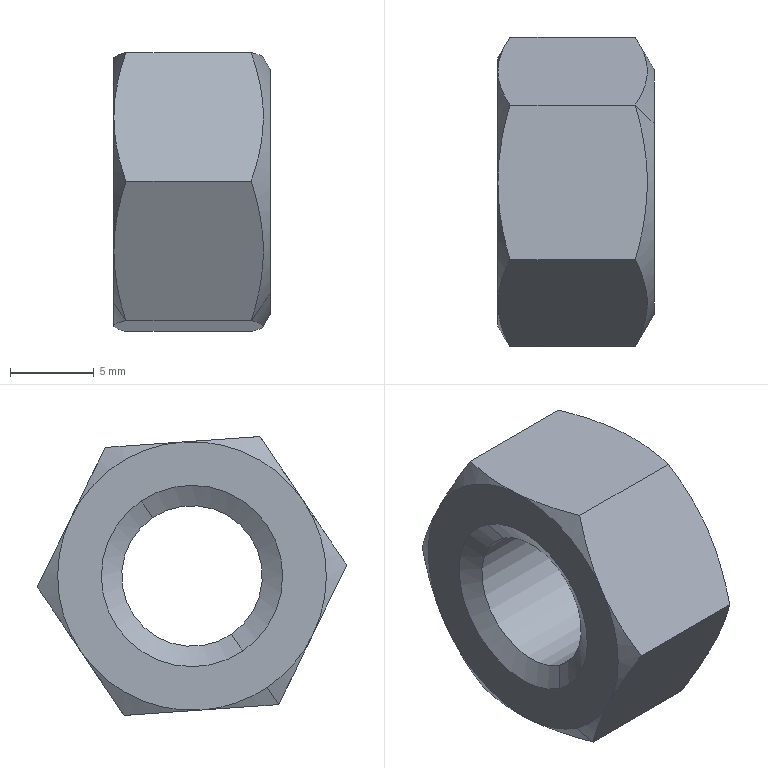Part | NX | features BREP 1 | 1 solid | 23 faces | box 9.3 x 18.43 x 16.607 mm | volume 1512 mm3 | cone 13 | plane 8 | cylinder 2 | commonest cylinder face diameters 8.376 x2
STEP:
#1=CARTESIAN_POINT('',(711.535,38.26,-40.972));
#2=VERTEX_POINT('',#1);
#3=CARTESIAN_POINT('',(711.535,33.574,-47.915));
#4=VERTEX_POINT('',#3);
#5=CARTESIAN_POINT('',(711.535,35.917,-44.443));
#6=DIRECTION('',(1.,0.,0.));
#7=DIRECTION('',(0.,-0.5594,-0.8289));
#8=AXIS2_PLACEMENT_3D('',#5,#6,#7);
#9=CIRCLE('',#8,4.188);
#10=EDGE_CURVE('',#2,#4,#9,.T.);
#11=ORIENTED_EDGE('',*,*,#10,.F.);
#12=CARTESIAN_POINT('',(711.845,38.433,-40.715));
#13=VERTEX_POINT('',#12);
#14=CARTESIAN_POINT('',(711.535,38.26,-40.972));
#15=DIRECTION('',(0.7071,0.3956,0.5861));
#16=VECTOR('',#15,1000.);
#17=LINE('',#14,#16);
#18=EDGE_CURVE('',#13,#2,#17,.F.);
#19=ORIENTED_EDGE('',*,*,#18,.F.);
#20=CARTESIAN_POINT('',(711.845,33.401,-48.172));
#21=VERTEX_POINT('',#20);
#22=CARTESIAN_POINT('',(711.845,35.917,-44.443));
#23=DIRECTION('',(-1.,0.,0.));
#24=DIRECTION('',(0.,-0.5594,-0.8289));
#25=AXIS2_PLACEMENT_3D('',#22,#23,#24);
#26=CIRCLE('',#25,4.498);
#27=EDGE_CURVE('',#21,#13,#26,.T.);
#28=ORIENTED_EDGE('',*,*,#27,.F.);
#29=CARTESIAN_POINT('',(711.535,33.574,-47.915));
#30=DIRECTION('',(0.7071,-0.3956,-0.5861));
#31=VECTOR('',#30,1000.);
#32=LINE('',#29,#31);
#33=EDGE_CURVE('',#21,#4,#32,.F.);
#34=ORIENTED_EDGE('',*,*,#33,.T.);
#35=EDGE_LOOP('',(#11,#19,#28,#34));
#36=FACE_BOUND('',#35,.T.);
#37=CARTESIAN_POINT('',(711.535,35.917,-44.443));
#38=DIRECTION('',(1.,0.,0.));
#39=DIRECTION('',(0.,0.5594,0.8289));
#40=AXIS2_PLACEMENT_3D('',#37,#38,#39);
#41=CONICAL_SURFACE('',#40,4.188,0.7854);
#42=ADVANCED_FACE('',(#36),#41,.F.);
#43=CARTESIAN_POINT('',(711.845,40.001,-38.392));
#44=VERTEX_POINT('',#43);
#45=CARTESIAN_POINT('',(711.845,31.834,-50.494));
#46=VERTEX_POINT('',#45);
#47=CARTESIAN_POINT('',(711.845,35.917,-44.443));
#48=DIRECTION('',(-1.,0.,0.));
#49=DIRECTION('',(0.,0.5594,0.8289));
#50=AXIS2_PLACEMENT_3D('',#47,#48,#49);
#51=CIRCLE('',#50,7.3);
#52=EDGE_CURVE('',#44,#46,#51,.T.);
#53=ORIENTED_EDGE('',*,*,#52,.T.);
#54=CARTESIAN_POINT('',(710.726,30.75,-52.1));
#55=VERTEX_POINT('',#54);
#56=CARTESIAN_POINT('',(710.726,30.75,-52.1));
#57=DIRECTION('',(-0.5,-0.4845,-0.7178));
#58=VECTOR('',#57,1000.);
#59=LINE('',#56,#58);
#60=EDGE_CURVE('',#46,#55,#59,.T.);
#61=ORIENTED_EDGE('',*,*,#60,.T.);
#62=CARTESIAN_POINT('',(710.726,39.965,-52.747));
#63=VERTEX_POINT('',#62);
#64=CARTESIAN_POINT('',(710.726,39.965,-52.747));
#65=CARTESIAN_POINT('',(711.162,38.46,-52.641));
#66=CARTESIAN_POINT('',(711.72,35.374,-52.425));
#67=CARTESIAN_POINT('',(711.162,32.256,-52.206));
#68=CARTESIAN_POINT('',(710.726,30.75,-52.1));
#69=B_SPLINE_CURVE_WITH_KNOTS('',3,(#64,#65,#66,#67,#68),.UNSPECIFIED.,.F.,.F.,(4,1,4),(0.,0.004665,0.009329),.UNSPECIFIED.);
#70=EDGE_CURVE('',#63,#55,#69,.T.);
#71=ORIENTED_EDGE('',*,*,#70,.F.);
#72=CARTESIAN_POINT('',(710.726,45.132,-45.09));
#73=VERTEX_POINT('',#72);
#74=CARTESIAN_POINT('',(710.726,45.132,-45.09));
#75=CARTESIAN_POINT('',(711.162,44.288,-46.34));
#76=CARTESIAN_POINT('',(711.72,42.558,-48.905));
#77=CARTESIAN_POINT('',(711.162,40.809,-51.495));
#78=CARTESIAN_POINT('',(710.726,39.965,-52.747));
#79=B_SPLINE_CURVE_WITH_KNOTS('',3,(#74,#75,#76,#77,#78),.UNSPECIFIED.,.F.,.F.,(4,1,4),(0.,0.004665,0.009329),.UNSPECIFIED.);
#80=EDGE_CURVE('',#73,#63,#79,.T.);
#81=ORIENTED_EDGE('',*,*,#80,.F.);
#82=CARTESIAN_POINT('',(710.726,41.085,-36.786));
#83=VERTEX_POINT('',#82);
#84=CARTESIAN_POINT('',(710.726,41.085,-36.786));
#85=CARTESIAN_POINT('',(711.162,41.746,-38.142));
#86=CARTESIAN_POINT('',(711.72,43.101,-40.923));
#87=CARTESIAN_POINT('',(711.162,44.47,-43.732));
#88=CARTESIAN_POINT('',(710.726,45.132,-45.09));
#89=B_SPLINE_CURVE_WITH_KNOTS('',3,(#84,#85,#86,#87,#88),.UNSPECIFIED.,.F.,.F.,(4,1,4),(0.,0.004665,0.009329),.UNSPECIFIED.);
#90=EDGE_CURVE('',#83,#73,#89,.T.);
#91=ORIENTED_EDGE('',*,*,#90,.F.);
#92=CARTESIAN_POINT('',(710.726,41.085,-36.786));
#93=DIRECTION('',(-0.5,0.4845,0.7178));
#94=VECTOR('',#93,1000.);
#95=LINE('',#92,#94);
#96=EDGE_CURVE('',#44,#83,#95,.T.);
#97=ORIENTED_EDGE('',*,*,#96,.F.);
#98=EDGE_LOOP('',(#53,#61,#71,#81,#91,#97));
#99=FACE_BOUND('',#98,.T.);
#100=CARTESIAN_POINT('',(710.726,35.917,-44.443));
#101=DIRECTION('',(-1.,0.,0.));
#102=DIRECTION('',(0.,-0.5594,-0.8289));
#103=AXIS2_PLACEMENT_3D('',#100,#101,#102);
#104=CONICAL_SURFACE('',#103,9.238,1.047);
#105=ADVANCED_FACE('',(#99),#104,.T.);
#106=CARTESIAN_POINT('',(703.245,38.26,-40.972));
#107=VERTEX_POINT('',#106);
#108=CARTESIAN_POINT('',(703.245,33.574,-47.915));
#109=VERTEX_POINT('',#108);
#110=CARTESIAN_POINT('',(703.245,35.917,-44.443));
#111=DIRECTION('',(1.,0.,0.));
#112=DIRECTION('',(0.,-0.5594,-0.8289));
#113=AXIS2_PLACEMENT_3D('',#110,#111,#112);
#114=CIRCLE('',#113,4.188);
#115=EDGE_CURVE('',#107,#109,#114,.T.);
#116=ORIENTED_EDGE('',*,*,#115,.T.);
#117=CARTESIAN_POINT('',(702.545,32.896,-48.919));
#118=VERTEX_POINT('',#117);
#119=CARTESIAN_POINT('',(703.245,33.574,-47.915));
#120=DIRECTION('',(-0.5,-0.4845,-0.7178));
#121=VECTOR('',#120,1000.);
#122=LINE('',#119,#121);
#123=EDGE_CURVE('',#109,#118,#122,.T.);
#124=ORIENTED_EDGE('',*,*,#123,.T.);
#125=CARTESIAN_POINT('',(702.545,38.938,-39.967));
#126=VERTEX_POINT('',#125);
#127=CARTESIAN_POINT('',(702.545,35.917,-44.443));
#128=DIRECTION('',(1.,0.,0.));
#129=DIRECTION('',(0.,-0.5594,-0.8289));
#130=AXIS2_PLACEMENT_3D('',#127,#128,#129);
#131=CIRCLE('',#130,5.4);
#132=EDGE_CURVE('',#126,#118,#131,.T.);
#133=ORIENTED_EDGE('',*,*,#132,.F.);
#134=CARTESIAN_POINT('',(703.245,38.26,-40.972));
#135=DIRECTION('',(-0.5,0.4845,0.7178));
#136=VECTOR('',#135,1000.);
#137=LINE('',#134,#136);
#138=EDGE_CURVE('',#107,#126,#137,.T.);
#139=ORIENTED_EDGE('',*,*,#138,.F.);
#140=EDGE_LOOP('',(#116,#124,#133,#139));
#141=FACE_BOUND('',#140,.T.);
#142=CARTESIAN_POINT('',(703.245,35.917,-44.443));
#143=DIRECTION('',(-1.,0.,0.));
#144=DIRECTION('',(0.,-0.5594,-0.8289));
#145=AXIS2_PLACEMENT_3D('',#142,#143,#144);
#146=CONICAL_SURFACE('',#145,4.188,1.047);
#147=ADVANCED_FACE('',(#141),#146,.F.);
#148=CARTESIAN_POINT('',(702.545,28.726,-47.948));
#149=VERTEX_POINT('',#148);
#150=CARTESIAN_POINT('',(702.545,31.442,-51.074));
#151=VERTEX_POINT('',#150);
#152=CARTESIAN_POINT('',(702.545,35.917,-44.443));
#153=DIRECTION('',(1.,0.,0.));
#154=DIRECTION('',(0.,-0.5594,-0.8289));
#155=AXIS2_PLACEMENT_3D('',#152,#153,#154);
#156=CIRCLE('',#155,8.);
#157=EDGE_CURVE('',#149,#151,#156,.T.);
#158=ORIENTED_EDGE('',*,*,#157,.T.);
#159=CARTESIAN_POINT('',(703.26,30.75,-52.1));
#160=VERTEX_POINT('',#159);
#161=CARTESIAN_POINT('',(703.26,30.75,-52.1));
#162=DIRECTION('',(0.5,-0.4845,-0.7178));
#163=VECTOR('',#162,1000.);
#164=LINE('',#161,#163);
#165=EDGE_CURVE('',#151,#160,#164,.T.);
#166=ORIENTED_EDGE('',*,*,#165,.T.);
#167=CARTESIAN_POINT('',(702.545,28.726,-47.948));
#168=CARTESIAN_POINT('',(702.545,29.417,-49.366));
#169=CARTESIAN_POINT('',(702.824,30.088,-50.744));
#170=CARTESIAN_POINT('',(703.26,30.75,-52.1));
#171=B_SPLINE_CURVE_WITH_KNOTS('',3,(#167,#168,#169,#170),.UNSPECIFIED.,.F.,.F.,(4,4),(0.,0.004674),.UNSPECIFIED.);
#172=EDGE_CURVE('',#149,#160,#171,.T.);
#173=ORIENTED_EDGE('',*,*,#172,.F.);
#174=EDGE_LOOP('',(#158,#166,#173));
#175=FACE_BOUND('',#174,.T.);
#176=CARTESIAN_POINT('',(703.26,35.917,-44.443));
#177=DIRECTION('',(1.,0.,0.));
#178=DIRECTION('',(0.,0.5594,0.8289));
#179=AXIS2_PLACEMENT_3D('',#176,#177,#178);
#180=CONICAL_SURFACE('',#179,9.238,1.047);
#181=ADVANCED_FACE('',(#175),#180,.T.);
#182=ORIENTED_EDGE('',*,*,#115,.F.);
#183=CARTESIAN_POINT('',(702.545,38.26,-40.972));
#184=DIRECTION('',(1.,0.,0.));
#185=VECTOR('',#184,1000.);
#186=LINE('',#183,#185);
#187=EDGE_CURVE('',#2,#107,#186,.F.);
#188=ORIENTED_EDGE('',*,*,#187,.F.);
#189=ORIENTED_EDGE('',*,*,#10,.T.);
#190=CARTESIAN_POINT('',(702.545,33.574,-47.915));
#191=DIRECTION('',(1.,0.,0.));
#192=VECTOR('',#191,1000.);
#193=LINE('',#190,#192);
#194=EDGE_CURVE('',#4,#109,#193,.F.);
#195=ORIENTED_EDGE('',*,*,#194,.T.);
#196=EDGE_LOOP('',(#182,#188,#189,#195));
#197=FACE_BOUND('',#196,.T.);
#198=CARTESIAN_POINT('',(702.545,35.917,-44.443));
#199=DIRECTION('',(1.,0.,0.));
#200=DIRECTION('',(0.,0.5594,0.8289));
#201=AXIS2_PLACEMENT_3D('',#198,#199,#200);
#202=CYLINDRICAL_SURFACE('',#201,4.188);
#203=ADVANCED_FACE('',(#197),#202,.F.);
#204=CARTESIAN_POINT('',(703.26,26.702,-43.797));
#205=VERTEX_POINT('',#204);
#206=CARTESIAN_POINT('',(710.726,26.702,-43.797));
#207=VERTEX_POINT('',#206);
#208=CARTESIAN_POINT('',(702.545,26.702,-43.797));
#209=DIRECTION('',(1.,0.,0.));
#210=VECTOR('',#209,1000.);
#211=LINE('',#208,#210);
#212=EDGE_CURVE('',#205,#207,#211,.T.);
#213=ORIENTED_EDGE('',*,*,#212,.T.);
#214=CARTESIAN_POINT('',(710.726,31.87,-36.14));
#215=VERTEX_POINT('',#214);
#216=CARTESIAN_POINT('',(710.726,26.702,-43.797));
#217=CARTESIAN_POINT('',(711.162,27.546,-42.546));
#218=CARTESIAN_POINT('',(711.72,29.277,-39.982));
#219=CARTESIAN_POINT('',(711.162,31.025,-37.391));
#220=CARTESIAN_POINT('',(710.726,31.87,-36.14));
#221=B_SPLINE_CURVE_WITH_KNOTS('',3,(#216,#217,#218,#219,#220),.UNSPECIFIED.,.F.,.F.,(4,1,4),(0.,0.004665,0.009329),.UNSPECIFIED.);
#222=EDGE_CURVE('',#207,#215,#221,.T.);
#223=ORIENTED_EDGE('',*,*,#222,.T.);
#224=CARTESIAN_POINT('',(703.26,31.87,-36.14));
#225=VERTEX_POINT('',#224);
#226=CARTESIAN_POINT('',(702.545,31.87,-36.14));
#227=DIRECTION('',(1.,0.,0.));
#228=VECTOR('',#227,1000.);
#229=LINE('',#226,#228);
#230=EDGE_CURVE('',#225,#215,#229,.T.);
#231=ORIENTED_EDGE('',*,*,#230,.F.);
#232=CARTESIAN_POINT('',(702.545,29.286,-39.968));
#233=VERTEX_POINT('',#232);
#234=CARTESIAN_POINT('',(703.26,31.87,-36.14));
#235=CARTESIAN_POINT('',(702.824,31.026,-37.39));
#236=CARTESIAN_POINT('',(702.545,30.168,-38.661));
#237=CARTESIAN_POINT('',(702.545,29.286,-39.968));
#238=B_SPLINE_CURVE_WITH_KNOTS('',3,(#234,#235,#236,#237),.UNSPECIFIED.,.F.,.F.,(4,4),(0.,0.004674),.UNSPECIFIED.);
#239=EDGE_CURVE('',#225,#233,#238,.T.);
#240=ORIENTED_EDGE('',*,*,#239,.T.);
#241=CARTESIAN_POINT('',(702.545,29.286,-39.968));
#242=CARTESIAN_POINT('',(702.545,28.404,-41.275));
#243=CARTESIAN_POINT('',(702.824,27.546,-42.546));
#244=CARTESIAN_POINT('',(703.26,26.702,-43.797));
#245=B_SPLINE_CURVE_WITH_KNOTS('',3,(#241,#242,#243,#244),.UNSPECIFIED.,.F.,.F.,(4,4),(0.,0.004674),.UNSPECIFIED.);
#246=EDGE_CURVE('',#233,#205,#245,.T.);
#247=ORIENTED_EDGE('',*,*,#246,.T.);
#248=EDGE_LOOP('',(#213,#223,#231,#240,#247));
#249=FACE_BOUND('',#248,.T.);
#250=CARTESIAN_POINT('',(702.545,31.87,-36.14));
#251=DIRECTION('',(0.,-0.8289,0.5594));
#252=DIRECTION('',(1.,0.,0.));
#253=AXIS2_PLACEMENT_3D('',#250,#251,#252);
#254=PLANE('',#253);
#255=ADVANCED_FACE('',(#249),#254,.T.);
#256=ORIENTED_EDGE('',*,*,#230,.T.);
#257=CARTESIAN_POINT('',(710.726,31.87,-36.14));
#258=CARTESIAN_POINT('',(711.162,33.374,-36.245));
#259=CARTESIAN_POINT('',(711.72,36.461,-36.462));
#260=CARTESIAN_POINT('',(711.162,39.578,-36.681));
#261=CARTESIAN_POINT('',(710.726,41.085,-36.786));
#262=B_SPLINE_CURVE_WITH_KNOTS('',3,(#257,#258,#259,#260,#261),.UNSPECIFIED.,.F.,.F.,(4,1,4),(0.,0.004665,0.009329),.UNSPECIFIED.);
#263=EDGE_CURVE('',#215,#83,#262,.T.);
#264=ORIENTED_EDGE('',*,*,#263,.T.);
#265=CARTESIAN_POINT('',(703.26,41.085,-36.786));
#266=VERTEX_POINT('',#265);
#267=CARTESIAN_POINT('',(702.545,41.085,-36.786));
#268=DIRECTION('',(1.,0.,0.));
#269=VECTOR('',#268,1000.);
#270=LINE('',#267,#269);
#271=EDGE_CURVE('',#266,#83,#270,.T.);
#272=ORIENTED_EDGE('',*,*,#271,.F.);
#273=CARTESIAN_POINT('',(702.545,36.477,-36.463));
#274=VERTEX_POINT('',#273);
#275=CARTESIAN_POINT('',(703.26,41.085,-36.786));
#276=CARTESIAN_POINT('',(702.824,39.579,-36.681));
#277=CARTESIAN_POINT('',(702.545,38.05,-36.573));
#278=CARTESIAN_POINT('',(702.545,36.477,-36.463));
#279=B_SPLINE_CURVE_WITH_KNOTS('',3,(#275,#276,#277,#278),.UNSPECIFIED.,.F.,.F.,(4,4),(0.,0.004674),.UNSPECIFIED.);
#280=EDGE_CURVE('',#266,#274,#279,.T.);
#281=ORIENTED_EDGE('',*,*,#280,.T.);
#282=CARTESIAN_POINT('',(702.545,36.477,-36.463));
#283=CARTESIAN_POINT('',(702.545,34.905,-36.353));
#284=CARTESIAN_POINT('',(702.824,33.375,-36.245));
#285=CARTESIAN_POINT('',(703.26,31.87,-36.14));
#286=B_SPLINE_CURVE_WITH_KNOTS('',3,(#282,#283,#284,#285),.UNSPECIFIED.,.F.,.F.,(4,4),(0.,0.004674),.UNSPECIFIED.);
#287=EDGE_CURVE('',#274,#225,#286,.T.);
#288=ORIENTED_EDGE('',*,*,#287,.T.);
#289=EDGE_LOOP('',(#256,#264,#272,#281,#288));
#290=FACE_BOUND('',#289,.T.);
#291=CARTESIAN_POINT('',(702.545,41.085,-36.786));
#292=DIRECTION('',(0.,0.07,0.9975));
#293=DIRECTION('',(0.,0.9975,-0.07));
#294=AXIS2_PLACEMENT_3D('',#291,#292,#293);
#295=PLANE('',#294);
#296=ADVANCED_FACE('',(#290),#295,.T.);
#297=ORIENTED_EDGE('',*,*,#271,.T.);
#298=ORIENTED_EDGE('',*,*,#90,.T.);
#299=CARTESIAN_POINT('',(703.26,45.132,-45.09));
#300=VERTEX_POINT('',#299);
#301=CARTESIAN_POINT('',(702.545,45.132,-45.09));
#302=DIRECTION('',(1.,0.,0.));
#303=VECTOR('',#302,1000.);
#304=LINE('',#301,#303);
#305=EDGE_CURVE('',#300,#73,#304,.T.);
#306=ORIENTED_EDGE('',*,*,#305,.F.);
#307=CARTESIAN_POINT('',(702.545,43.108,-40.938));
#308=VERTEX_POINT('',#307);
#309=CARTESIAN_POINT('',(703.26,45.132,-45.09));
#310=CARTESIAN_POINT('',(702.824,44.471,-43.733));
#311=CARTESIAN_POINT('',(702.545,43.799,-42.355));
#312=CARTESIAN_POINT('',(702.545,43.108,-40.938));
#313=B_SPLINE_CURVE_WITH_KNOTS('',3,(#309,#310,#311,#312),.UNSPECIFIED.,.F.,.F.,(4,4),(0.,0.004674),.UNSPECIFIED.);
#314=EDGE_CURVE('',#300,#308,#313,.T.);
#315=ORIENTED_EDGE('',*,*,#314,.T.);
#316=CARTESIAN_POINT('',(702.545,43.108,-40.938));
#317=CARTESIAN_POINT('',(702.545,42.418,-39.521));
#318=CARTESIAN_POINT('',(702.824,41.746,-38.143));
#319=CARTESIAN_POINT('',(703.26,41.085,-36.786));
#320=B_SPLINE_CURVE_WITH_KNOTS('',3,(#316,#317,#318,#319),.UNSPECIFIED.,.F.,.F.,(4,4),(0.,0.004674),.UNSPECIFIED.);
#321=EDGE_CURVE('',#308,#266,#320,.T.);
#322=ORIENTED_EDGE('',*,*,#321,.T.);
#323=EDGE_LOOP('',(#297,#298,#306,#315,#322));
#324=FACE_BOUND('',#323,.T.);
#325=CARTESIAN_POINT('',(702.545,45.132,-45.09));
#326=DIRECTION('',(0.,0.8989,0.4381));
#327=DIRECTION('',(0.,0.4381,-0.8989));
#328=AXIS2_PLACEMENT_3D('',#325,#326,#327);
#329=PLANE('',#328);
#330=ADVANCED_FACE('',(#324),#329,.T.);
#331=ORIENTED_EDGE('',*,*,#305,.T.);
#332=ORIENTED_EDGE('',*,*,#80,.T.);
#333=CARTESIAN_POINT('',(703.26,39.965,-52.747));
#334=VERTEX_POINT('',#333);
#335=CARTESIAN_POINT('',(702.545,39.965,-52.747));
#336=DIRECTION('',(1.,0.,0.));
#337=VECTOR('',#336,1000.);
#338=LINE('',#335,#337);
#339=EDGE_CURVE('',#334,#63,#338,.T.);
#340=ORIENTED_EDGE('',*,*,#339,.F.);
#341=CARTESIAN_POINT('',(702.545,42.548,-48.918));
#342=VERTEX_POINT('',#341);
#343=CARTESIAN_POINT('',(703.26,39.965,-52.747));
#344=CARTESIAN_POINT('',(702.824,40.809,-51.496));
#345=CARTESIAN_POINT('',(702.545,41.667,-50.225));
#346=CARTESIAN_POINT('',(702.545,42.548,-48.918));
#347=B_SPLINE_CURVE_WITH_KNOTS('',3,(#343,#344,#345,#346),.UNSPECIFIED.,.F.,.F.,(4,4),(0.,0.004674),.UNSPECIFIED.);
#348=EDGE_CURVE('',#334,#342,#347,.T.);
#349=ORIENTED_EDGE('',*,*,#348,.T.);
#350=CARTESIAN_POINT('',(702.545,42.548,-48.918));
#351=CARTESIAN_POINT('',(702.545,43.43,-47.612));
#352=CARTESIAN_POINT('',(702.824,44.288,-46.341));
#353=CARTESIAN_POINT('',(703.26,45.132,-45.09));
#354=B_SPLINE_CURVE_WITH_KNOTS('',3,(#350,#351,#352,#353),.UNSPECIFIED.,.F.,.F.,(4,4),(0.,0.004674),.UNSPECIFIED.);
#355=EDGE_CURVE('',#342,#300,#354,.T.);
#356=ORIENTED_EDGE('',*,*,#355,.T.);
#357=EDGE_LOOP('',(#331,#332,#340,#349,#356));
#358=FACE_BOUND('',#357,.T.);
#359=CARTESIAN_POINT('',(702.545,39.965,-52.747));
#360=DIRECTION('',(0.,0.8289,-0.5594));
#361=DIRECTION('',(0.,-0.5594,-0.8289));
#362=AXIS2_PLACEMENT_3D('',#359,#360,#361);
#363=PLANE('',#362);
#364=ADVANCED_FACE('',(#358),#363,.T.);
#365=ORIENTED_EDGE('',*,*,#339,.T.);
#366=ORIENTED_EDGE('',*,*,#70,.T.);
#367=CARTESIAN_POINT('',(702.545,30.75,-52.1));
#368=DIRECTION('',(1.,0.,0.));
#369=VECTOR('',#368,1000.);
#370=LINE('',#367,#369);
#371=EDGE_CURVE('',#160,#55,#370,.T.);
#372=ORIENTED_EDGE('',*,*,#371,.F.);
#373=CARTESIAN_POINT('',(702.545,35.357,-52.424));
#374=VERTEX_POINT('',#373);
#375=CARTESIAN_POINT('',(703.26,30.75,-52.1));
#376=CARTESIAN_POINT('',(702.824,32.255,-52.206));
#377=CARTESIAN_POINT('',(702.545,33.785,-52.313));
#378=CARTESIAN_POINT('',(702.545,35.357,-52.424));
#379=B_SPLINE_CURVE_WITH_KNOTS('',3,(#375,#376,#377,#378),.UNSPECIFIED.,.F.,.F.,(4,4),(0.,0.004674),.UNSPECIFIED.);
#380=EDGE_CURVE('',#160,#374,#379,.T.);
#381=ORIENTED_EDGE('',*,*,#380,.T.);
#382=CARTESIAN_POINT('',(702.545,35.357,-52.424));
#383=CARTESIAN_POINT('',(702.545,36.93,-52.534));
#384=CARTESIAN_POINT('',(702.824,38.459,-52.641));
#385=CARTESIAN_POINT('',(703.26,39.965,-52.747));
#386=B_SPLINE_CURVE_WITH_KNOTS('',3,(#382,#383,#384,#385),.UNSPECIFIED.,.F.,.F.,(4,4),(0.,0.004674),.UNSPECIFIED.);
#387=EDGE_CURVE('',#374,#334,#386,.T.);
#388=ORIENTED_EDGE('',*,*,#387,.T.);
#389=EDGE_LOOP('',(#365,#366,#372,#381,#388));
#390=FACE_BOUND('',#389,.T.);
#391=CARTESIAN_POINT('',(702.545,30.75,-52.1));
#392=DIRECTION('',(0.,-0.07,-0.9975));
#393=DIRECTION('',(0.,-0.9975,0.07));
#394=AXIS2_PLACEMENT_3D('',#391,#392,#393);
#395=PLANE('',#394);
#396=ADVANCED_FACE('',(#390),#395,.T.);
#397=ORIENTED_EDGE('',*,*,#371,.T.);
#398=CARTESIAN_POINT('',(710.726,30.75,-52.1));
#399=CARTESIAN_POINT('',(711.162,30.089,-50.744));
#400=CARTESIAN_POINT('',(711.72,28.733,-47.964));
#401=CARTESIAN_POINT('',(711.162,27.364,-45.154));
#402=CARTESIAN_POINT('',(710.726,26.702,-43.797));
#403=B_SPLINE_CURVE_WITH_KNOTS('',3,(#398,#399,#400,#401,#402),.UNSPECIFIED.,.F.,.F.,(4,1,4),(0.,0.004665,0.009329),.UNSPECIFIED.);
#404=EDGE_CURVE('',#55,#207,#403,.T.);
#405=ORIENTED_EDGE('',*,*,#404,.T.);
#406=ORIENTED_EDGE('',*,*,#212,.F.);
#407=CARTESIAN_POINT('',(703.26,26.702,-43.797));
#408=CARTESIAN_POINT('',(702.824,27.363,-45.153));
#409=CARTESIAN_POINT('',(702.545,28.035,-46.531));
#410=CARTESIAN_POINT('',(702.545,28.726,-47.948));
#411=B_SPLINE_CURVE_WITH_KNOTS('',3,(#407,#408,#409,#410),.UNSPECIFIED.,.F.,.F.,(4,4),(0.,0.004674),.UNSPECIFIED.);
#412=EDGE_CURVE('',#205,#149,#411,.T.);
#413=ORIENTED_EDGE('',*,*,#412,.T.);
#414=ORIENTED_EDGE('',*,*,#172,.T.);
#415=EDGE_LOOP('',(#397,#405,#406,#413,#414));
#416=FACE_BOUND('',#415,.T.);
#417=CARTESIAN_POINT('',(702.545,26.702,-43.797));
#418=DIRECTION('',(0.,-0.8989,-0.4381));
#419=DIRECTION('',(0.,-0.4381,0.8989));
#420=AXIS2_PLACEMENT_3D('',#417,#418,#419);
#421=PLANE('',#420);
#422=ADVANCED_FACE('',(#416),#421,.T.);
#423=ORIENTED_EDGE('',*,*,#27,.T.);
#424=CARTESIAN_POINT('',(711.845,35.917,-44.443));
#425=DIRECTION('',(-1.,0.,0.));
#426=DIRECTION('',(0.,-0.5594,-0.8289));
#427=AXIS2_PLACEMENT_3D('',#424,#425,#426);
#428=CIRCLE('',#427,4.498);
#429=EDGE_CURVE('',#13,#21,#428,.T.);
#430=ORIENTED_EDGE('',*,*,#429,.T.);
#431=EDGE_LOOP('',(#423,#430));
#432=FACE_BOUND('',#431,.T.);
#433=ORIENTED_EDGE('',*,*,#52,.F.);
#434=CARTESIAN_POINT('',(711.845,35.917,-44.443));
#435=DIRECTION('',(-1.,0.,0.));
#436=DIRECTION('',(0.,0.5594,0.8289));
#437=AXIS2_PLACEMENT_3D('',#434,#435,#436);
#438=CIRCLE('',#437,7.3);
#439=EDGE_CURVE('',#46,#44,#438,.T.);
#440=ORIENTED_EDGE('',*,*,#439,.F.);
#441=EDGE_LOOP('',(#433,#440));
#442=FACE_BOUND('',#441,.T.);
#443=CARTESIAN_POINT('',(711.845,26.702,-43.797));
#444=DIRECTION('',(1.,0.,0.));
#445=DIRECTION('',(0.,0.5594,0.8289));
#446=AXIS2_PLACEMENT_3D('',#443,#444,#445);
#447=PLANE('',#446);
#448=ADVANCED_FACE('',(#432,#442),#447,.T.);
#449=ORIENTED_EDGE('',*,*,#132,.T.);
#450=CARTESIAN_POINT('',(702.545,35.917,-44.443));
#451=DIRECTION('',(1.,0.,0.));
#452=DIRECTION('',(0.,-0.5594,-0.8289));
#453=AXIS2_PLACEMENT_3D('',#450,#451,#452);
#454=CIRCLE('',#453,5.4);
#455=EDGE_CURVE('',#118,#126,#454,.T.);
#456=ORIENTED_EDGE('',*,*,#455,.T.);
#457=EDGE_LOOP('',(#449,#456));
#458=FACE_BOUND('',#457,.T.);
#459=CARTESIAN_POINT('',(702.545,35.917,-44.443));
#460=DIRECTION('',(1.,0.,0.));
#461=DIRECTION('',(0.,-0.5594,-0.8289));
#462=AXIS2_PLACEMENT_3D('',#459,#460,#461);
#463=CIRCLE('',#462,8.);
#464=EDGE_CURVE('',#374,#342,#463,.T.);
#465=ORIENTED_EDGE('',*,*,#464,.F.);
#466=CARTESIAN_POINT('',(702.545,35.917,-44.443));
#467=DIRECTION('',(1.,0.,0.));
#468=DIRECTION('',(0.,-0.5594,-0.8289));
#469=AXIS2_PLACEMENT_3D('',#466,#467,#468);
#470=CIRCLE('',#469,8.);
#471=EDGE_CURVE('',#151,#374,#470,.T.);
#472=ORIENTED_EDGE('',*,*,#471,.F.);
#473=ORIENTED_EDGE('',*,*,#157,.F.);
#474=CARTESIAN_POINT('',(702.545,35.917,-44.443));
#475=DIRECTION('',(1.,0.,0.));
#476=DIRECTION('',(0.,-0.5594,-0.8289));
#477=AXIS2_PLACEMENT_3D('',#474,#475,#476);
#478=CIRCLE('',#477,8.);
#479=EDGE_CURVE('',#233,#149,#478,.T.);
#480=ORIENTED_EDGE('',*,*,#479,.F.);
#481=CARTESIAN_POINT('',(702.545,35.917,-44.443));
#482=DIRECTION('',(1.,0.,0.));
#483=DIRECTION('',(0.,-0.5594,-0.8289));
#484=AXIS2_PLACEMENT_3D('',#481,#482,#483);
#485=CIRCLE('',#484,8.);
#486=EDGE_CURVE('',#274,#233,#485,.T.);
#487=ORIENTED_EDGE('',*,*,#486,.F.);
#488=CARTESIAN_POINT('',(702.545,35.917,-44.443));
#489=DIRECTION('',(1.,0.,0.));
#490=DIRECTION('',(0.,-0.5594,-0.8289));
#491=AXIS2_PLACEMENT_3D('',#488,#489,#490);
#492=CIRCLE('',#491,8.);
#493=EDGE_CURVE('',#308,#274,#492,.T.);
#494=ORIENTED_EDGE('',*,*,#493,.F.);
#495=CARTESIAN_POINT('',(702.545,35.917,-44.443));
#496=DIRECTION('',(1.,0.,0.));
#497=DIRECTION('',(0.,-0.5594,-0.8289));
#498=AXIS2_PLACEMENT_3D('',#495,#496,#497);
#499=CIRCLE('',#498,8.);
#500=EDGE_CURVE('',#342,#308,#499,.T.);
#501=ORIENTED_EDGE('',*,*,#500,.F.);
#502=EDGE_LOOP('',(#465,#472,#473,#480,#487,#494,#501));
#503=FACE_BOUND('',#502,.T.);
#504=CARTESIAN_POINT('',(702.545,26.702,-43.797));
#505=DIRECTION('',(1.,0.,0.));
#506=DIRECTION('',(0.,0.5594,0.8289));
#507=AXIS2_PLACEMENT_3D('',#504,#505,#506);
#508=PLANE('',#507);
#509=ADVANCED_FACE('',(#458,#503),#508,.F.);
#510=ORIENTED_EDGE('',*,*,#187,.T.);
#511=CARTESIAN_POINT('',(703.245,35.917,-44.443));
#512=DIRECTION('',(1.,0.,0.));
#513=DIRECTION('',(0.,-0.5594,-0.8289));
#514=AXIS2_PLACEMENT_3D('',#511,#512,#513);
#515=CIRCLE('',#514,4.188);
#516=EDGE_CURVE('',#109,#107,#515,.T.);
#517=ORIENTED_EDGE('',*,*,#516,.F.);
#518=ORIENTED_EDGE('',*,*,#194,.F.);
#519=CARTESIAN_POINT('',(711.535,35.917,-44.443));
#520=DIRECTION('',(1.,0.,0.));
#521=DIRECTION('',(0.,-0.5594,-0.8289));
#522=AXIS2_PLACEMENT_3D('',#519,#520,#521);
#523=CIRCLE('',#522,4.188);
#524=EDGE_CURVE('',#4,#2,#523,.T.);
#525=ORIENTED_EDGE('',*,*,#524,.T.);
#526=EDGE_LOOP('',(#510,#517,#518,#525));
#527=FACE_BOUND('',#526,.T.);
#528=CARTESIAN_POINT('',(702.545,35.917,-44.443));
#529=DIRECTION('',(1.,0.,0.));
#530=DIRECTION('',(0.,0.5594,0.8289));
#531=AXIS2_PLACEMENT_3D('',#528,#529,#530);
#532=CYLINDRICAL_SURFACE('',#531,4.188);
#533=ADVANCED_FACE('',(#527),#532,.F.);
#534=ORIENTED_EDGE('',*,*,#165,.F.);
#535=ORIENTED_EDGE('',*,*,#471,.T.);
#536=ORIENTED_EDGE('',*,*,#380,.F.);
#537=EDGE_LOOP('',(#534,#535,#536));
#538=FACE_BOUND('',#537,.T.);
#539=CARTESIAN_POINT('',(703.26,35.917,-44.443));
#540=DIRECTION('',(1.,0.,0.));
#541=DIRECTION('',(0.,0.5594,0.8289));
#542=AXIS2_PLACEMENT_3D('',#539,#540,#541);
#543=CONICAL_SURFACE('',#542,9.238,1.047);
#544=ADVANCED_FACE('',(#538),#543,.T.);
#545=ORIENTED_EDGE('',*,*,#479,.T.);
#546=ORIENTED_EDGE('',*,*,#412,.F.);
#547=ORIENTED_EDGE('',*,*,#246,.F.);
#548=EDGE_LOOP('',(#545,#546,#547));
#549=FACE_BOUND('',#548,.T.);
#550=CARTESIAN_POINT('',(703.26,35.917,-44.443));
#551=DIRECTION('',(1.,0.,0.));
#552=DIRECTION('',(0.,0.5594,0.8289));
#553=AXIS2_PLACEMENT_3D('',#550,#551,#552);
#554=CONICAL_SURFACE('',#553,9.238,1.047);
#555=ADVANCED_FACE('',(#549),#554,.T.);
#556=ORIENTED_EDGE('',*,*,#486,.T.);
#557=ORIENTED_EDGE('',*,*,#239,.F.);
#558=ORIENTED_EDGE('',*,*,#287,.F.);
#559=EDGE_LOOP('',(#556,#557,#558));
#560=FACE_BOUND('',#559,.T.);
#561=CARTESIAN_POINT('',(703.26,35.917,-44.443));
#562=DIRECTION('',(1.,0.,0.));
#563=DIRECTION('',(0.,0.5594,0.8289));
#564=AXIS2_PLACEMENT_3D('',#561,#562,#563);
#565=CONICAL_SURFACE('',#564,9.238,1.047);
#566=ADVANCED_FACE('',(#560),#565,.T.);
#567=ORIENTED_EDGE('',*,*,#493,.T.);
#568=ORIENTED_EDGE('',*,*,#280,.F.);
#569=ORIENTED_EDGE('',*,*,#321,.F.);
#570=EDGE_LOOP('',(#567,#568,#569));
#571=FACE_BOUND('',#570,.T.);
#572=CARTESIAN_POINT('',(703.26,35.917,-44.443));
#573=DIRECTION('',(1.,0.,0.));
#574=DIRECTION('',(0.,0.5594,0.8289));
#575=AXIS2_PLACEMENT_3D('',#572,#573,#574);
#576=CONICAL_SURFACE('',#575,9.238,1.047);
#577=ADVANCED_FACE('',(#571),#576,.T.);
#578=ORIENTED_EDGE('',*,*,#355,.F.);
#579=ORIENTED_EDGE('',*,*,#500,.T.);
#580=ORIENTED_EDGE('',*,*,#314,.F.);
#581=EDGE_LOOP('',(#578,#579,#580));
#582=FACE_BOUND('',#581,.T.);
#583=CARTESIAN_POINT('',(703.26,35.917,-44.443));
#584=DIRECTION('',(1.,0.,0.));
#585=DIRECTION('',(0.,0.5594,0.8289));
#586=AXIS2_PLACEMENT_3D('',#583,#584,#585);
#587=CONICAL_SURFACE('',#586,9.238,1.047);
#588=ADVANCED_FACE('',(#582),#587,.T.);
#589=ORIENTED_EDGE('',*,*,#387,.F.);
#590=ORIENTED_EDGE('',*,*,#464,.T.);
#591=ORIENTED_EDGE('',*,*,#348,.F.);
#592=EDGE_LOOP('',(#589,#590,#591));
#593=FACE_BOUND('',#592,.T.);
#594=CARTESIAN_POINT('',(703.26,35.917,-44.443));
#595=DIRECTION('',(1.,0.,0.));
#596=DIRECTION('',(0.,0.5594,0.8289));
#597=AXIS2_PLACEMENT_3D('',#594,#595,#596);
#598=CONICAL_SURFACE('',#597,9.238,1.047);
#599=ADVANCED_FACE('',(#593),#598,.T.);
#600=ORIENTED_EDGE('',*,*,#123,.F.);
#601=ORIENTED_EDGE('',*,*,#516,.T.);
#602=ORIENTED_EDGE('',*,*,#138,.T.);
#603=ORIENTED_EDGE('',*,*,#455,.F.);
#604=EDGE_LOOP('',(#600,#601,#602,#603));
#605=FACE_BOUND('',#604,.T.);
#606=CARTESIAN_POINT('',(703.245,35.917,-44.443));
#607=DIRECTION('',(-1.,0.,0.));
#608=DIRECTION('',(0.,-0.5594,-0.8289));
#609=AXIS2_PLACEMENT_3D('',#606,#607,#608);
#610=CONICAL_SURFACE('',#609,4.188,1.047);
#611=ADVANCED_FACE('',(#605),#610,.F.);
#612=ORIENTED_EDGE('',*,*,#60,.F.);
#613=ORIENTED_EDGE('',*,*,#439,.T.);
#614=ORIENTED_EDGE('',*,*,#96,.T.);
#615=ORIENTED_EDGE('',*,*,#263,.F.);
#616=ORIENTED_EDGE('',*,*,#222,.F.);
#617=ORIENTED_EDGE('',*,*,#404,.F.);
#618=EDGE_LOOP('',(#612,#613,#614,#615,#616,#617));
#619=FACE_BOUND('',#618,.T.);
#620=CARTESIAN_POINT('',(710.726,35.917,-44.443));
#621=DIRECTION('',(-1.,0.,0.));
#622=DIRECTION('',(0.,-0.5594,-0.8289));
#623=AXIS2_PLACEMENT_3D('',#620,#621,#622);
#624=CONICAL_SURFACE('',#623,9.238,1.047);
#625=ADVANCED_FACE('',(#619),#624,.T.);
#626=ORIENTED_EDGE('',*,*,#18,.T.);
#627=ORIENTED_EDGE('',*,*,#524,.F.);
#628=ORIENTED_EDGE('',*,*,#33,.F.);
#629=ORIENTED_EDGE('',*,*,#429,.F.);
#630=EDGE_LOOP('',(#626,#627,#628,#629));
#631=FACE_BOUND('',#630,.T.);
#632=CARTESIAN_POINT('',(711.535,35.917,-44.443));
#633=DIRECTION('',(1.,0.,0.));
#634=DIRECTION('',(0.,0.5594,0.8289));
#635=AXIS2_PLACEMENT_3D('',#632,#633,#634);
#636=CONICAL_SURFACE('',#635,4.188,0.7854);
#637=ADVANCED_FACE('',(#631),#636,.F.);
#638=CLOSED_SHELL('',(#42,#105,#147,#181,#203,#255,#296,#330,#364,#396,#422,#448,#509,#533,#544,#555,#566,#577,#588,#599,#611,#625,#637));
#639=MANIFOLD_SOLID_BREP('',#638);
#640=(LENGTH_UNIT()NAMED_UNIT(*)SI_UNIT(.MILLI.,.METRE.));
#641=UNCERTAINTY_MEASURE_WITH_UNIT(LENGTH_MEASURE(0.0508),#640,'','');
#642=(NAMED_UNIT(*)PLANE_ANGLE_UNIT()SI_UNIT($,.RADIAN.));
#643=(NAMED_UNIT(*)SI_UNIT($,.STERADIAN.)SOLID_ANGLE_UNIT());
#644=(GEOMETRIC_REPRESENTATION_CONTEXT(3)GLOBAL_UNCERTAINTY_ASSIGNED_CONTEXT((#641))GLOBAL_UNIT_ASSIGNED_CONTEXT((#640,#642,#643))REPRESENTATION_CONTEXT('',''));
#645=ADVANCED_BREP_SHAPE_REPRESENTATION('',(#639),#644);